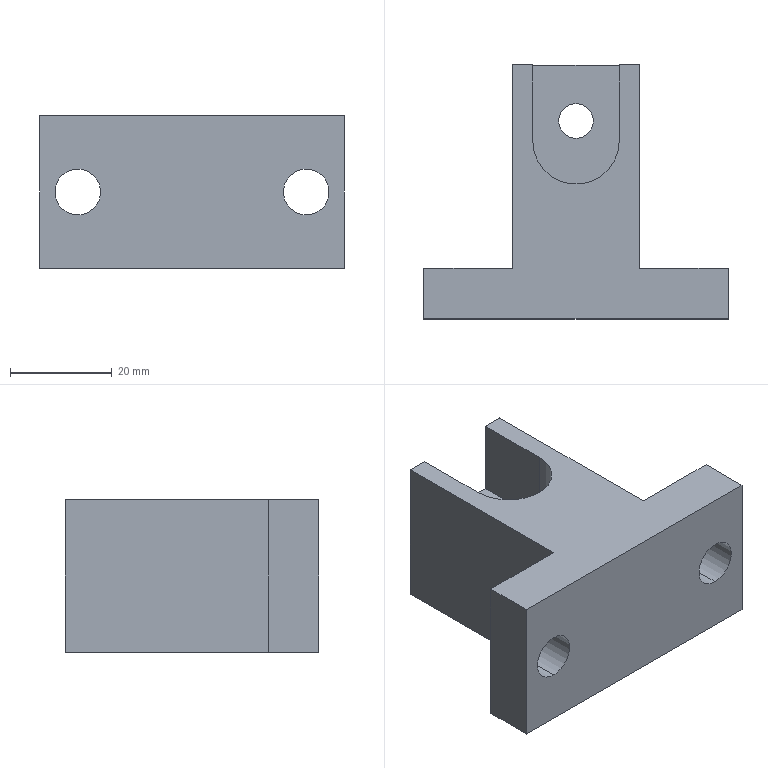Part | SolidWorks | features 3DProfileFeature 2, HoleWzd 2, Extrusion 1, ICE 1 | 1 solid | 20 faces | box 60 x 50 x 30 mm | volume 40656 mm3 | plane 13 | cylinder 7 | commonest cylinder face diameters 9 x4 6.8 x2 17 x1
STEP:
#1=CARTESIAN_POINT('',(26.6,39.,15.));
#2=VERTEX_POINT('',#1);
#3=CARTESIAN_POINT('',(33.4,39.,15.));
#4=VERTEX_POINT('',#3);
#5=CARTESIAN_POINT('',(30.,39.,15.));
#6=DIRECTION('',(0.,0.,1.));
#7=DIRECTION('',(1.,0.,0.));
#8=AXIS2_PLACEMENT_3D('',#5,#6,#7);
#9=CIRCLE('',#8,3.4);
#10=EDGE_CURVE('',#2,#4,#9,.T.);
#11=ORIENTED_EDGE('',*,*,#10,.T.);
#12=CARTESIAN_POINT('',(33.4,39.,0.));
#13=VERTEX_POINT('',#12);
#14=CARTESIAN_POINT('',(33.4,39.,0.));
#15=DIRECTION('',(0.,0.,-1.));
#16=VECTOR('',#15,1000.);
#17=LINE('',#14,#16);
#18=EDGE_CURVE('',#4,#13,#17,.T.);
#19=ORIENTED_EDGE('',*,*,#18,.T.);
#20=CARTESIAN_POINT('',(26.6,39.,0.));
#21=VERTEX_POINT('',#20);
#22=CARTESIAN_POINT('',(30.,39.,0.));
#23=DIRECTION('',(0.,0.,-1.));
#24=DIRECTION('',(-1.,0.,0.));
#25=AXIS2_PLACEMENT_3D('',#22,#23,#24);
#26=CIRCLE('',#25,3.4);
#27=EDGE_CURVE('',#13,#21,#26,.T.);
#28=ORIENTED_EDGE('',*,*,#27,.T.);
#29=CARTESIAN_POINT('',(26.6,39.,0.));
#30=DIRECTION('',(0.,0.,-1.));
#31=VECTOR('',#30,1000.);
#32=LINE('',#29,#31);
#33=EDGE_CURVE('',#2,#21,#32,.T.);
#34=ORIENTED_EDGE('',*,*,#33,.F.);
#35=EDGE_LOOP('',(#11,#19,#28,#34));
#36=FACE_OUTER_BOUND('',#35,.T.);
#37=CARTESIAN_POINT('',(30.,39.,0.));
#38=DIRECTION('',(0.,0.,-1.));
#39=DIRECTION('',(-1.,0.,0.));
#40=AXIS2_PLACEMENT_3D('',#37,#38,#39);
#41=CYLINDRICAL_SURFACE('',#40,3.4);
#42=ADVANCED_FACE('',(#36),#41,.F.);
#43=CARTESIAN_POINT('',(7.5,10.,19.5));
#44=VERTEX_POINT('',#43);
#45=CARTESIAN_POINT('',(7.5,10.,10.5));
#46=VERTEX_POINT('',#45);
#47=CARTESIAN_POINT('',(7.5,10.,15.));
#48=DIRECTION('',(0.,-1.,0.));
#49=DIRECTION('',(0.,0.,-1.));
#50=AXIS2_PLACEMENT_3D('',#47,#48,#49);
#51=CIRCLE('',#50,4.5);
#52=EDGE_CURVE('',#44,#46,#51,.T.);
#53=ORIENTED_EDGE('',*,*,#52,.F.);
#54=CARTESIAN_POINT('',(7.5,0.,19.5));
#55=VERTEX_POINT('',#54);
#56=CARTESIAN_POINT('',(7.5,0.,19.5));
#57=DIRECTION('',(0.,-1.,0.));
#58=VECTOR('',#57,1000.);
#59=LINE('',#56,#58);
#60=EDGE_CURVE('',#44,#55,#59,.T.);
#61=ORIENTED_EDGE('',*,*,#60,.T.);
#62=CARTESIAN_POINT('',(7.5,0.,10.5));
#63=VERTEX_POINT('',#62);
#64=CARTESIAN_POINT('',(7.5,0.,15.));
#65=DIRECTION('',(0.,-1.,0.));
#66=DIRECTION('',(0.,0.,-1.));
#67=AXIS2_PLACEMENT_3D('',#64,#65,#66);
#68=CIRCLE('',#67,4.5);
#69=EDGE_CURVE('',#55,#63,#68,.T.);
#70=ORIENTED_EDGE('',*,*,#69,.T.);
#71=CARTESIAN_POINT('',(7.5,0.,10.5));
#72=DIRECTION('',(0.,-1.,0.));
#73=VECTOR('',#72,1000.);
#74=LINE('',#71,#73);
#75=EDGE_CURVE('',#46,#63,#74,.T.);
#76=ORIENTED_EDGE('',*,*,#75,.F.);
#77=EDGE_LOOP('',(#53,#61,#70,#76));
#78=FACE_OUTER_BOUND('',#77,.T.);
#79=CARTESIAN_POINT('',(7.5,0.,15.));
#80=DIRECTION('',(0.,-1.,0.));
#81=DIRECTION('',(0.,0.,-1.));
#82=AXIS2_PLACEMENT_3D('',#79,#80,#81);
#83=CYLINDRICAL_SURFACE('',#82,4.5);
#84=ADVANCED_FACE('',(#78),#83,.F.);
#85=CARTESIAN_POINT('',(52.5,10.,19.5));
#86=VERTEX_POINT('',#85);
#87=CARTESIAN_POINT('',(52.5,10.,10.5));
#88=VERTEX_POINT('',#87);
#89=CARTESIAN_POINT('',(52.5,10.,15.));
#90=DIRECTION('',(0.,-1.,0.));
#91=DIRECTION('',(0.,0.,-1.));
#92=AXIS2_PLACEMENT_3D('',#89,#90,#91);
#93=CIRCLE('',#92,4.5);
#94=EDGE_CURVE('',#86,#88,#93,.T.);
#95=ORIENTED_EDGE('',*,*,#94,.F.);
#96=CARTESIAN_POINT('',(52.5,0.,19.5));
#97=VERTEX_POINT('',#96);
#98=CARTESIAN_POINT('',(52.5,0.,19.5));
#99=DIRECTION('',(0.,-1.,0.));
#100=VECTOR('',#99,1000.);
#101=LINE('',#98,#100);
#102=EDGE_CURVE('',#86,#97,#101,.T.);
#103=ORIENTED_EDGE('',*,*,#102,.T.);
#104=CARTESIAN_POINT('',(52.5,0.,10.5));
#105=VERTEX_POINT('',#104);
#106=CARTESIAN_POINT('',(52.5,0.,15.));
#107=DIRECTION('',(0.,-1.,0.));
#108=DIRECTION('',(0.,0.,-1.));
#109=AXIS2_PLACEMENT_3D('',#106,#107,#108);
#110=CIRCLE('',#109,4.5);
#111=EDGE_CURVE('',#97,#105,#110,.T.);
#112=ORIENTED_EDGE('',*,*,#111,.T.);
#113=CARTESIAN_POINT('',(52.5,0.,10.5));
#114=DIRECTION('',(0.,-1.,0.));
#115=VECTOR('',#114,1000.);
#116=LINE('',#113,#115);
#117=EDGE_CURVE('',#88,#105,#116,.T.);
#118=ORIENTED_EDGE('',*,*,#117,.F.);
#119=EDGE_LOOP('',(#95,#103,#112,#118));
#120=FACE_OUTER_BOUND('',#119,.T.);
#121=CARTESIAN_POINT('',(52.5,0.,15.));
#122=DIRECTION('',(0.,-1.,0.));
#123=DIRECTION('',(0.,0.,-1.));
#124=AXIS2_PLACEMENT_3D('',#121,#122,#123);
#125=CYLINDRICAL_SURFACE('',#124,4.5);
#126=ADVANCED_FACE('',(#120),#125,.F.);
#127=CARTESIAN_POINT('',(7.5,0.,15.));
#128=DIRECTION('',(0.,-1.,0.));
#129=DIRECTION('',(0.,0.,-1.));
#130=AXIS2_PLACEMENT_3D('',#127,#128,#129);
#131=CIRCLE('',#130,4.5);
#132=EDGE_CURVE('',#63,#55,#131,.T.);
#133=ORIENTED_EDGE('',*,*,#132,.F.);
#134=ORIENTED_EDGE('',*,*,#69,.F.);
#135=EDGE_LOOP('',(#133,#134));
#136=FACE_BOUND('',#135,.T.);
#137=CARTESIAN_POINT('',(52.5,0.,15.));
#138=DIRECTION('',(0.,-1.,0.));
#139=DIRECTION('',(0.,0.,-1.));
#140=AXIS2_PLACEMENT_3D('',#137,#138,#139);
#141=CIRCLE('',#140,4.5);
#142=EDGE_CURVE('',#105,#97,#141,.T.);
#143=ORIENTED_EDGE('',*,*,#142,.F.);
#144=ORIENTED_EDGE('',*,*,#111,.F.);
#145=EDGE_LOOP('',(#143,#144));
#146=FACE_BOUND('',#145,.T.);
#147=CARTESIAN_POINT('',(0.,0.,0.));
#148=VERTEX_POINT('',#147);
#149=CARTESIAN_POINT('',(60.,0.,0.));
#150=VERTEX_POINT('',#149);
#151=CARTESIAN_POINT('',(60.,0.,0.));
#152=DIRECTION('',(1.,0.,0.));
#153=VECTOR('',#152,1000.);
#154=LINE('',#151,#153);
#155=EDGE_CURVE('',#148,#150,#154,.T.);
#156=ORIENTED_EDGE('',*,*,#155,.T.);
#157=CARTESIAN_POINT('',(60.,0.,30.));
#158=VERTEX_POINT('',#157);
#159=CARTESIAN_POINT('',(60.,0.,30.));
#160=DIRECTION('',(0.,0.,-1.));
#161=VECTOR('',#160,1000.);
#162=LINE('',#159,#161);
#163=EDGE_CURVE('',#158,#150,#162,.T.);
#164=ORIENTED_EDGE('',*,*,#163,.F.);
#165=CARTESIAN_POINT('',(0.,0.,30.));
#166=VERTEX_POINT('',#165);
#167=CARTESIAN_POINT('',(60.,0.,30.));
#168=DIRECTION('',(1.,0.,0.));
#169=VECTOR('',#168,1000.);
#170=LINE('',#167,#169);
#171=EDGE_CURVE('',#166,#158,#170,.T.);
#172=ORIENTED_EDGE('',*,*,#171,.F.);
#173=CARTESIAN_POINT('',(0.,0.,30.));
#174=DIRECTION('',(0.,0.,-1.));
#175=VECTOR('',#174,1000.);
#176=LINE('',#173,#175);
#177=EDGE_CURVE('',#166,#148,#176,.T.);
#178=ORIENTED_EDGE('',*,*,#177,.T.);
#179=EDGE_LOOP('',(#156,#164,#172,#178));
#180=FACE_OUTER_BOUND('',#179,.T.);
#181=CARTESIAN_POINT('',(60.,0.,30.));
#182=DIRECTION('',(0.,1.,0.));
#183=DIRECTION('',(-1.,0.,0.));
#184=AXIS2_PLACEMENT_3D('',#181,#182,#183);
#185=PLANE('',#184);
#186=ADVANCED_FACE('',(#136,#146,#180),#185,.F.);
#187=CARTESIAN_POINT('',(60.,10.,0.));
#188=VERTEX_POINT('',#187);
#189=CARTESIAN_POINT('',(60.,10.,0.));
#190=DIRECTION('',(0.,1.,0.));
#191=VECTOR('',#190,1000.);
#192=LINE('',#189,#191);
#193=EDGE_CURVE('',#150,#188,#192,.T.);
#194=ORIENTED_EDGE('',*,*,#193,.T.);
#195=CARTESIAN_POINT('',(60.,10.,30.));
#196=VERTEX_POINT('',#195);
#197=CARTESIAN_POINT('',(60.,10.,30.));
#198=DIRECTION('',(0.,0.,-1.));
#199=VECTOR('',#198,1000.);
#200=LINE('',#197,#199);
#201=EDGE_CURVE('',#196,#188,#200,.T.);
#202=ORIENTED_EDGE('',*,*,#201,.F.);
#203=CARTESIAN_POINT('',(60.,10.,30.));
#204=DIRECTION('',(0.,1.,0.));
#205=VECTOR('',#204,1000.);
#206=LINE('',#203,#205);
#207=EDGE_CURVE('',#158,#196,#206,.T.);
#208=ORIENTED_EDGE('',*,*,#207,.F.);
#209=ORIENTED_EDGE('',*,*,#163,.T.);
#210=EDGE_LOOP('',(#194,#202,#208,#209));
#211=FACE_OUTER_BOUND('',#210,.T.);
#212=CARTESIAN_POINT('',(60.,10.,30.));
#213=DIRECTION('',(-1.,0.,0.));
#214=DIRECTION('',(0.,0.,1.));
#215=AXIS2_PLACEMENT_3D('',#212,#213,#214);
#216=PLANE('',#215);
#217=ADVANCED_FACE('',(#211),#216,.F.);
#218=CARTESIAN_POINT('',(52.5,10.,15.));
#219=DIRECTION('',(0.,-1.,0.));
#220=DIRECTION('',(0.,0.,-1.));
#221=AXIS2_PLACEMENT_3D('',#218,#219,#220);
#222=CIRCLE('',#221,4.5);
#223=EDGE_CURVE('',#88,#86,#222,.T.);
#224=ORIENTED_EDGE('',*,*,#223,.T.);
#225=ORIENTED_EDGE('',*,*,#94,.T.);
#226=EDGE_LOOP('',(#224,#225));
#227=FACE_BOUND('',#226,.T.);
#228=CARTESIAN_POINT('',(42.5,10.,0.));
#229=VERTEX_POINT('',#228);
#230=CARTESIAN_POINT('',(42.5,10.,0.));
#231=DIRECTION('',(-1.,0.,0.));
#232=VECTOR('',#231,1000.);
#233=LINE('',#230,#232);
#234=EDGE_CURVE('',#188,#229,#233,.T.);
#235=ORIENTED_EDGE('',*,*,#234,.T.);
#236=CARTESIAN_POINT('',(42.5,10.,30.));
#237=VERTEX_POINT('',#236);
#238=CARTESIAN_POINT('',(42.5,10.,30.));
#239=DIRECTION('',(0.,0.,-1.));
#240=VECTOR('',#239,1000.);
#241=LINE('',#238,#240);
#242=EDGE_CURVE('',#237,#229,#241,.T.);
#243=ORIENTED_EDGE('',*,*,#242,.F.);
#244=CARTESIAN_POINT('',(42.5,10.,30.));
#245=DIRECTION('',(-1.,0.,0.));
#246=VECTOR('',#245,1000.);
#247=LINE('',#244,#246);
#248=EDGE_CURVE('',#196,#237,#247,.T.);
#249=ORIENTED_EDGE('',*,*,#248,.F.);
#250=ORIENTED_EDGE('',*,*,#201,.T.);
#251=EDGE_LOOP('',(#235,#243,#249,#250));
#252=FACE_OUTER_BOUND('',#251,.T.);
#253=CARTESIAN_POINT('',(42.5,10.,30.));
#254=DIRECTION('',(0.,-1.,0.));
#255=DIRECTION('',(0.,0.,-1.));
#256=AXIS2_PLACEMENT_3D('',#253,#254,#255);
#257=PLANE('',#256);
#258=ADVANCED_FACE('',(#227,#252),#257,.F.);
#259=CARTESIAN_POINT('',(42.5,50.,0.));
#260=VERTEX_POINT('',#259);
#261=CARTESIAN_POINT('',(42.5,50.,0.));
#262=DIRECTION('',(0.,1.,0.));
#263=VECTOR('',#262,1000.);
#264=LINE('',#261,#263);
#265=EDGE_CURVE('',#229,#260,#264,.T.);
#266=ORIENTED_EDGE('',*,*,#265,.T.);
#267=CARTESIAN_POINT('',(42.5,50.,30.));
#268=VERTEX_POINT('',#267);
#269=CARTESIAN_POINT('',(42.5,50.,30.));
#270=DIRECTION('',(0.,0.,-1.));
#271=VECTOR('',#270,1000.);
#272=LINE('',#269,#271);
#273=EDGE_CURVE('',#268,#260,#272,.T.);
#274=ORIENTED_EDGE('',*,*,#273,.F.);
#275=CARTESIAN_POINT('',(42.5,50.,30.));
#276=DIRECTION('',(0.,1.,0.));
#277=VECTOR('',#276,1000.);
#278=LINE('',#275,#277);
#279=EDGE_CURVE('',#237,#268,#278,.T.);
#280=ORIENTED_EDGE('',*,*,#279,.F.);
#281=ORIENTED_EDGE('',*,*,#242,.T.);
#282=EDGE_LOOP('',(#266,#274,#280,#281));
#283=FACE_OUTER_BOUND('',#282,.T.);
#284=CARTESIAN_POINT('',(42.5,50.,30.));
#285=DIRECTION('',(-1.,0.,0.));
#286=DIRECTION('',(0.,0.,1.));
#287=AXIS2_PLACEMENT_3D('',#284,#285,#286);
#288=PLANE('',#287);
#289=ADVANCED_FACE('',(#283),#288,.F.);
#290=CARTESIAN_POINT('',(38.5,50.,15.));
#291=VERTEX_POINT('',#290);
#292=CARTESIAN_POINT('',(21.5,50.,15.));
#293=VERTEX_POINT('',#292);
#294=CARTESIAN_POINT('',(17.5,50.,15.));
#295=DIRECTION('',(-1.,0.,0.));
#296=VECTOR('',#295,1000.);
#297=LINE('',#294,#296);
#298=EDGE_CURVE('',#291,#293,#297,.T.);
#299=ORIENTED_EDGE('',*,*,#298,.F.);
#300=CARTESIAN_POINT('',(38.5,50.,30.));
#301=VERTEX_POINT('',#300);
#302=CARTESIAN_POINT('',(38.5,50.,15.));
#303=DIRECTION('',(0.,0.,1.));
#304=VECTOR('',#303,1000.);
#305=LINE('',#302,#304);
#306=EDGE_CURVE('',#291,#301,#305,.T.);
#307=ORIENTED_EDGE('',*,*,#306,.T.);
#308=CARTESIAN_POINT('',(17.5,50.,30.));
#309=DIRECTION('',(-1.,0.,0.));
#310=VECTOR('',#309,1000.);
#311=LINE('',#308,#310);
#312=EDGE_CURVE('',#268,#301,#311,.T.);
#313=ORIENTED_EDGE('',*,*,#312,.F.);
#314=ORIENTED_EDGE('',*,*,#273,.T.);
#315=CARTESIAN_POINT('',(17.5,50.,0.));
#316=VERTEX_POINT('',#315);
#317=CARTESIAN_POINT('',(17.5,50.,0.));
#318=DIRECTION('',(-1.,0.,0.));
#319=VECTOR('',#318,1000.);
#320=LINE('',#317,#319);
#321=EDGE_CURVE('',#260,#316,#320,.T.);
#322=ORIENTED_EDGE('',*,*,#321,.T.);
#323=CARTESIAN_POINT('',(17.5,50.,30.));
#324=VERTEX_POINT('',#323);
#325=CARTESIAN_POINT('',(17.5,50.,30.));
#326=DIRECTION('',(0.,0.,-1.));
#327=VECTOR('',#326,1000.);
#328=LINE('',#325,#327);
#329=EDGE_CURVE('',#324,#316,#328,.T.);
#330=ORIENTED_EDGE('',*,*,#329,.F.);
#331=CARTESIAN_POINT('',(21.5,50.,30.));
#332=VERTEX_POINT('',#331);
#333=CARTESIAN_POINT('',(17.5,50.,30.));
#334=DIRECTION('',(-1.,0.,0.));
#335=VECTOR('',#334,1000.);
#336=LINE('',#333,#335);
#337=EDGE_CURVE('',#332,#324,#336,.T.);
#338=ORIENTED_EDGE('',*,*,#337,.F.);
#339=CARTESIAN_POINT('',(21.5,50.,15.));
#340=DIRECTION('',(0.,0.,1.));
#341=VECTOR('',#340,1000.);
#342=LINE('',#339,#341);
#343=EDGE_CURVE('',#293,#332,#342,.T.);
#344=ORIENTED_EDGE('',*,*,#343,.F.);
#345=EDGE_LOOP('',(#299,#307,#313,#314,#322,#330,#338,#344));
#346=FACE_OUTER_BOUND('',#345,.T.);
#347=CARTESIAN_POINT('',(17.5,50.,30.));
#348=DIRECTION('',(0.,-1.,0.));
#349=DIRECTION('',(0.,0.,-1.));
#350=AXIS2_PLACEMENT_3D('',#347,#348,#349);
#351=PLANE('',#350);
#352=ADVANCED_FACE('',(#346),#351,.F.);
#353=CARTESIAN_POINT('',(17.5,10.,0.));
#354=VERTEX_POINT('',#353);
#355=CARTESIAN_POINT('',(17.5,10.,0.));
#356=DIRECTION('',(0.,-1.,0.));
#357=VECTOR('',#356,1000.);
#358=LINE('',#355,#357);
#359=EDGE_CURVE('',#316,#354,#358,.T.);
#360=ORIENTED_EDGE('',*,*,#359,.T.);
#361=CARTESIAN_POINT('',(17.5,10.,30.));
#362=VERTEX_POINT('',#361);
#363=CARTESIAN_POINT('',(17.5,10.,30.));
#364=DIRECTION('',(0.,0.,-1.));
#365=VECTOR('',#364,1000.);
#366=LINE('',#363,#365);
#367=EDGE_CURVE('',#362,#354,#366,.T.);
#368=ORIENTED_EDGE('',*,*,#367,.F.);
#369=CARTESIAN_POINT('',(17.5,10.,30.));
#370=DIRECTION('',(0.,-1.,0.));
#371=VECTOR('',#370,1000.);
#372=LINE('',#369,#371);
#373=EDGE_CURVE('',#324,#362,#372,.T.);
#374=ORIENTED_EDGE('',*,*,#373,.F.);
#375=ORIENTED_EDGE('',*,*,#329,.T.);
#376=EDGE_LOOP('',(#360,#368,#374,#375));
#377=FACE_OUTER_BOUND('',#376,.T.);
#378=CARTESIAN_POINT('',(17.5,10.,30.));
#379=DIRECTION('',(1.,0.,0.));
#380=DIRECTION('',(0.,0.,-1.));
#381=AXIS2_PLACEMENT_3D('',#378,#379,#380);
#382=PLANE('',#381);
#383=ADVANCED_FACE('',(#377),#382,.F.);
#384=CARTESIAN_POINT('',(7.5,10.,15.));
#385=DIRECTION('',(0.,-1.,0.));
#386=DIRECTION('',(0.,0.,-1.));
#387=AXIS2_PLACEMENT_3D('',#384,#385,#386);
#388=CIRCLE('',#387,4.5);
#389=EDGE_CURVE('',#46,#44,#388,.T.);
#390=ORIENTED_EDGE('',*,*,#389,.T.);
#391=ORIENTED_EDGE('',*,*,#52,.T.);
#392=EDGE_LOOP('',(#390,#391));
#393=FACE_BOUND('',#392,.T.);
#394=CARTESIAN_POINT('',(0.,10.,0.));
#395=VERTEX_POINT('',#394);
#396=CARTESIAN_POINT('',(0.,10.,0.));
#397=DIRECTION('',(-1.,0.,0.));
#398=VECTOR('',#397,1000.);
#399=LINE('',#396,#398);
#400=EDGE_CURVE('',#354,#395,#399,.T.);
#401=ORIENTED_EDGE('',*,*,#400,.T.);
#402=CARTESIAN_POINT('',(0.,10.,30.));
#403=VERTEX_POINT('',#402);
#404=CARTESIAN_POINT('',(0.,10.,30.));
#405=DIRECTION('',(0.,0.,-1.));
#406=VECTOR('',#405,1000.);
#407=LINE('',#404,#406);
#408=EDGE_CURVE('',#403,#395,#407,.T.);
#409=ORIENTED_EDGE('',*,*,#408,.F.);
#410=CARTESIAN_POINT('',(0.,10.,30.));
#411=DIRECTION('',(-1.,0.,0.));
#412=VECTOR('',#411,1000.);
#413=LINE('',#410,#412);
#414=EDGE_CURVE('',#362,#403,#413,.T.);
#415=ORIENTED_EDGE('',*,*,#414,.F.);
#416=ORIENTED_EDGE('',*,*,#367,.T.);
#417=EDGE_LOOP('',(#401,#409,#415,#416));
#418=FACE_OUTER_BOUND('',#417,.T.);
#419=CARTESIAN_POINT('',(0.,10.,30.));
#420=DIRECTION('',(0.,-1.,0.));
#421=DIRECTION('',(0.,0.,-1.));
#422=AXIS2_PLACEMENT_3D('',#419,#420,#421);
#423=PLANE('',#422);
#424=ADVANCED_FACE('',(#393,#418),#423,.F.);
#425=CARTESIAN_POINT('',(0.,0.,0.));
#426=DIRECTION('',(0.,-1.,0.));
#427=VECTOR('',#426,1000.);
#428=LINE('',#425,#427);
#429=EDGE_CURVE('',#395,#148,#428,.T.);
#430=ORIENTED_EDGE('',*,*,#429,.T.);
#431=ORIENTED_EDGE('',*,*,#177,.F.);
#432=CARTESIAN_POINT('',(0.,0.,30.));
#433=DIRECTION('',(0.,-1.,0.));
#434=VECTOR('',#433,1000.);
#435=LINE('',#432,#434);
#436=EDGE_CURVE('',#403,#166,#435,.T.);
#437=ORIENTED_EDGE('',*,*,#436,.F.);
#438=ORIENTED_EDGE('',*,*,#408,.T.);
#439=EDGE_LOOP('',(#430,#431,#437,#438));
#440=FACE_OUTER_BOUND('',#439,.T.);
#441=CARTESIAN_POINT('',(0.,0.,30.));
#442=DIRECTION('',(1.,0.,0.));
#443=DIRECTION('',(0.,0.,-1.));
#444=AXIS2_PLACEMENT_3D('',#441,#442,#443);
#445=PLANE('',#444);
#446=ADVANCED_FACE('',(#440),#445,.F.);
#447=ORIENTED_EDGE('',*,*,#312,.T.);
#448=CARTESIAN_POINT('',(38.5,35.,30.));
#449=VERTEX_POINT('',#448);
#450=CARTESIAN_POINT('',(38.5,50.,30.));
#451=DIRECTION('',(0.,1.,0.));
#452=VECTOR('',#451,1000.);
#453=LINE('',#450,#452);
#454=EDGE_CURVE('',#449,#301,#453,.T.);
#455=ORIENTED_EDGE('',*,*,#454,.F.);
#456=CARTESIAN_POINT('',(21.5,35.,30.));
#457=VERTEX_POINT('',#456);
#458=CARTESIAN_POINT('',(30.,35.,30.));
#459=DIRECTION('',(0.,0.,1.));
#460=DIRECTION('',(1.,0.,0.));
#461=AXIS2_PLACEMENT_3D('',#458,#459,#460);
#462=CIRCLE('',#461,8.5);
#463=EDGE_CURVE('',#457,#449,#462,.T.);
#464=ORIENTED_EDGE('',*,*,#463,.F.);
#465=CARTESIAN_POINT('',(21.5,50.,30.));
#466=DIRECTION('',(0.,-1.,0.));
#467=VECTOR('',#466,1000.);
#468=LINE('',#465,#467);
#469=EDGE_CURVE('',#332,#457,#468,.T.);
#470=ORIENTED_EDGE('',*,*,#469,.F.);
#471=ORIENTED_EDGE('',*,*,#337,.T.);
#472=ORIENTED_EDGE('',*,*,#373,.T.);
#473=ORIENTED_EDGE('',*,*,#414,.T.);
#474=ORIENTED_EDGE('',*,*,#436,.T.);
#475=ORIENTED_EDGE('',*,*,#171,.T.);
#476=ORIENTED_EDGE('',*,*,#207,.T.);
#477=ORIENTED_EDGE('',*,*,#248,.T.);
#478=ORIENTED_EDGE('',*,*,#279,.T.);
#479=EDGE_LOOP('',(#447,#455,#464,#470,#471,#472,#473,#474,#475,#476,#477,#478));
#480=FACE_OUTER_BOUND('',#479,.T.);
#481=CARTESIAN_POINT('',(0.,0.,30.));
#482=DIRECTION('',(0.,0.,-1.));
#483=DIRECTION('',(-1.,0.,0.));
#484=AXIS2_PLACEMENT_3D('',#481,#482,#483);
#485=PLANE('',#484);
#486=ADVANCED_FACE('',(#480),#485,.F.);
#487=CARTESIAN_POINT('',(30.,39.,0.));
#488=DIRECTION('',(0.,0.,-1.));
#489=DIRECTION('',(-1.,0.,0.));
#490=AXIS2_PLACEMENT_3D('',#487,#488,#489);
#491=CIRCLE('',#490,3.4);
#492=EDGE_CURVE('',#21,#13,#491,.T.);
#493=ORIENTED_EDGE('',*,*,#492,.F.);
#494=ORIENTED_EDGE('',*,*,#27,.F.);
#495=EDGE_LOOP('',(#493,#494));
#496=FACE_BOUND('',#495,.T.);
#497=ORIENTED_EDGE('',*,*,#155,.F.);
#498=ORIENTED_EDGE('',*,*,#429,.F.);
#499=ORIENTED_EDGE('',*,*,#400,.F.);
#500=ORIENTED_EDGE('',*,*,#359,.F.);
#501=ORIENTED_EDGE('',*,*,#321,.F.);
#502=ORIENTED_EDGE('',*,*,#265,.F.);
#503=ORIENTED_EDGE('',*,*,#234,.F.);
#504=ORIENTED_EDGE('',*,*,#193,.F.);
#505=EDGE_LOOP('',(#497,#498,#499,#500,#501,#502,#503,#504));
#506=FACE_OUTER_BOUND('',#505,.T.);
#507=CARTESIAN_POINT('',(0.,0.,0.));
#508=DIRECTION('',(0.,0.,-1.));
#509=DIRECTION('',(-1.,0.,0.));
#510=AXIS2_PLACEMENT_3D('',#507,#508,#509);
#511=PLANE('',#510);
#512=ADVANCED_FACE('',(#496,#506),#511,.T.);
#513=ORIENTED_EDGE('',*,*,#10,.F.);
#514=CARTESIAN_POINT('',(30.,39.,15.));
#515=DIRECTION('',(0.,0.,1.));
#516=DIRECTION('',(1.,0.,0.));
#517=AXIS2_PLACEMENT_3D('',#514,#515,#516);
#518=CIRCLE('',#517,3.4);
#519=EDGE_CURVE('',#4,#2,#518,.T.);
#520=ORIENTED_EDGE('',*,*,#519,.F.);
#521=EDGE_LOOP('',(#513,#520));
#522=FACE_BOUND('',#521,.T.);
#523=ORIENTED_EDGE('',*,*,#298,.T.);
#524=CARTESIAN_POINT('',(21.5,35.,15.));
#525=VERTEX_POINT('',#524);
#526=CARTESIAN_POINT('',(21.5,50.,15.));
#527=DIRECTION('',(0.,-1.,0.));
#528=VECTOR('',#527,1000.);
#529=LINE('',#526,#528);
#530=EDGE_CURVE('',#293,#525,#529,.T.);
#531=ORIENTED_EDGE('',*,*,#530,.T.);
#532=CARTESIAN_POINT('',(38.5,35.,15.));
#533=VERTEX_POINT('',#532);
#534=CARTESIAN_POINT('',(30.,35.,15.));
#535=DIRECTION('',(0.,0.,1.));
#536=DIRECTION('',(1.,0.,0.));
#537=AXIS2_PLACEMENT_3D('',#534,#535,#536);
#538=CIRCLE('',#537,8.5);
#539=EDGE_CURVE('',#525,#533,#538,.T.);
#540=ORIENTED_EDGE('',*,*,#539,.T.);
#541=CARTESIAN_POINT('',(38.5,50.,15.));
#542=DIRECTION('',(0.,1.,0.));
#543=VECTOR('',#542,1000.);
#544=LINE('',#541,#543);
#545=EDGE_CURVE('',#533,#291,#544,.T.);
#546=ORIENTED_EDGE('',*,*,#545,.T.);
#547=EDGE_LOOP('',(#523,#531,#540,#546));
#548=FACE_OUTER_BOUND('',#547,.T.);
#549=CARTESIAN_POINT('',(30.,50.,15.));
#550=DIRECTION('',(0.,0.,1.));
#551=DIRECTION('',(1.,0.,0.));
#552=AXIS2_PLACEMENT_3D('',#549,#550,#551);
#553=PLANE('',#552);
#554=ADVANCED_FACE('',(#522,#548),#553,.T.);
#555=ORIENTED_EDGE('',*,*,#454,.T.);
#556=ORIENTED_EDGE('',*,*,#306,.F.);
#557=ORIENTED_EDGE('',*,*,#545,.F.);
#558=CARTESIAN_POINT('',(38.5,35.,15.));
#559=DIRECTION('',(0.,0.,1.));
#560=VECTOR('',#559,1000.);
#561=LINE('',#558,#560);
#562=EDGE_CURVE('',#533,#449,#561,.T.);
#563=ORIENTED_EDGE('',*,*,#562,.T.);
#564=EDGE_LOOP('',(#555,#556,#557,#563));
#565=FACE_OUTER_BOUND('',#564,.T.);
#566=CARTESIAN_POINT('',(38.5,50.,15.));
#567=DIRECTION('',(1.,0.,0.));
#568=DIRECTION('',(0.,1.,0.));
#569=AXIS2_PLACEMENT_3D('',#566,#567,#568);
#570=PLANE('',#569);
#571=ADVANCED_FACE('',(#565),#570,.F.);
#572=ORIENTED_EDGE('',*,*,#463,.T.);
#573=ORIENTED_EDGE('',*,*,#562,.F.);
#574=ORIENTED_EDGE('',*,*,#539,.F.);
#575=CARTESIAN_POINT('',(21.5,35.,15.));
#576=DIRECTION('',(0.,0.,1.));
#577=VECTOR('',#576,1000.);
#578=LINE('',#575,#577);
#579=EDGE_CURVE('',#525,#457,#578,.T.);
#580=ORIENTED_EDGE('',*,*,#579,.T.);
#581=EDGE_LOOP('',(#572,#573,#574,#580));
#582=FACE_OUTER_BOUND('',#581,.T.);
#583=CARTESIAN_POINT('',(30.,35.,15.));
#584=DIRECTION('',(0.,0.,1.));
#585=DIRECTION('',(1.,0.,0.));
#586=AXIS2_PLACEMENT_3D('',#583,#584,#585);
#587=CYLINDRICAL_SURFACE('',#586,8.5);
#588=ADVANCED_FACE('',(#582),#587,.F.);
#589=ORIENTED_EDGE('',*,*,#469,.T.);
#590=ORIENTED_EDGE('',*,*,#579,.F.);
#591=ORIENTED_EDGE('',*,*,#530,.F.);
#592=ORIENTED_EDGE('',*,*,#343,.T.);
#593=EDGE_LOOP('',(#589,#590,#591,#592));
#594=FACE_OUTER_BOUND('',#593,.T.);
#595=CARTESIAN_POINT('',(21.5,50.,15.));
#596=DIRECTION('',(-1.,0.,0.));
#597=DIRECTION('',(0.,-1.,0.));
#598=AXIS2_PLACEMENT_3D('',#595,#596,#597);
#599=PLANE('',#598);
#600=ADVANCED_FACE('',(#594),#599,.F.);
#601=ORIENTED_EDGE('',*,*,#102,.F.);
#602=ORIENTED_EDGE('',*,*,#223,.F.);
#603=ORIENTED_EDGE('',*,*,#117,.T.);
#604=ORIENTED_EDGE('',*,*,#142,.T.);
#605=EDGE_LOOP('',(#601,#602,#603,#604));
#606=FACE_OUTER_BOUND('',#605,.T.);
#607=CARTESIAN_POINT('',(52.5,0.,15.));
#608=DIRECTION('',(0.,-1.,0.));
#609=DIRECTION('',(0.,0.,-1.));
#610=AXIS2_PLACEMENT_3D('',#607,#608,#609);
#611=CYLINDRICAL_SURFACE('',#610,4.5);
#612=ADVANCED_FACE('',(#606),#611,.F.);
#613=ORIENTED_EDGE('',*,*,#60,.F.);
#614=ORIENTED_EDGE('',*,*,#389,.F.);
#615=ORIENTED_EDGE('',*,*,#75,.T.);
#616=ORIENTED_EDGE('',*,*,#132,.T.);
#617=EDGE_LOOP('',(#613,#614,#615,#616));
#618=FACE_OUTER_BOUND('',#617,.T.);
#619=CARTESIAN_POINT('',(7.5,0.,15.));
#620=DIRECTION('',(0.,-1.,0.));
#621=DIRECTION('',(0.,0.,-1.));
#622=AXIS2_PLACEMENT_3D('',#619,#620,#621);
#623=CYLINDRICAL_SURFACE('',#622,4.5);
#624=ADVANCED_FACE('',(#618),#623,.F.);
#625=ORIENTED_EDGE('',*,*,#18,.F.);
#626=ORIENTED_EDGE('',*,*,#519,.T.);
#627=ORIENTED_EDGE('',*,*,#33,.T.);
#628=ORIENTED_EDGE('',*,*,#492,.T.);
#629=EDGE_LOOP('',(#625,#626,#627,#628));
#630=FACE_OUTER_BOUND('',#629,.T.);
#631=CARTESIAN_POINT('',(30.,39.,0.));
#632=DIRECTION('',(0.,0.,-1.));
#633=DIRECTION('',(-1.,0.,0.));
#634=AXIS2_PLACEMENT_3D('',#631,#632,#633);
#635=CYLINDRICAL_SURFACE('',#634,3.4);
#636=ADVANCED_FACE('',(#630),#635,.F.);
#637=CLOSED_SHELL('',(#42,#84,#126,#186,#217,#258,#289,#352,#383,#424,#446,#486,#512,#554,#571,#588,#600,#612,#624,#636));
#638=MANIFOLD_SOLID_BREP('',#637);
#639=CARTESIAN_POINT('',(0.,0.,0.));
#640=DIRECTION('',(0.,0.,1.));
#641=DIRECTION('',(1.,0.,0.));
#642=AXIS2_PLACEMENT_3D('',#639,#640,#641);
#643=(LENGTH_UNIT()NAMED_UNIT(*)SI_UNIT(.MILLI.,.METRE.));
#644=UNCERTAINTY_MEASURE_WITH_UNIT(LENGTH_MEASURE(0.00001),#643,'','');
#645=(NAMED_UNIT(*)PLANE_ANGLE_UNIT()SI_UNIT($,.RADIAN.));
#646=(NAMED_UNIT(*)SI_UNIT($,.STERADIAN.)SOLID_ANGLE_UNIT());
#647=(GEOMETRIC_REPRESENTATION_CONTEXT(3)GLOBAL_UNCERTAINTY_ASSIGNED_CONTEXT((#644))GLOBAL_UNIT_ASSIGNED_CONTEXT((#643,#645,#646))REPRESENTATION_CONTEXT('',''));
#648=ADVANCED_BREP_SHAPE_REPRESENTATION('',(#638,#642),#647);